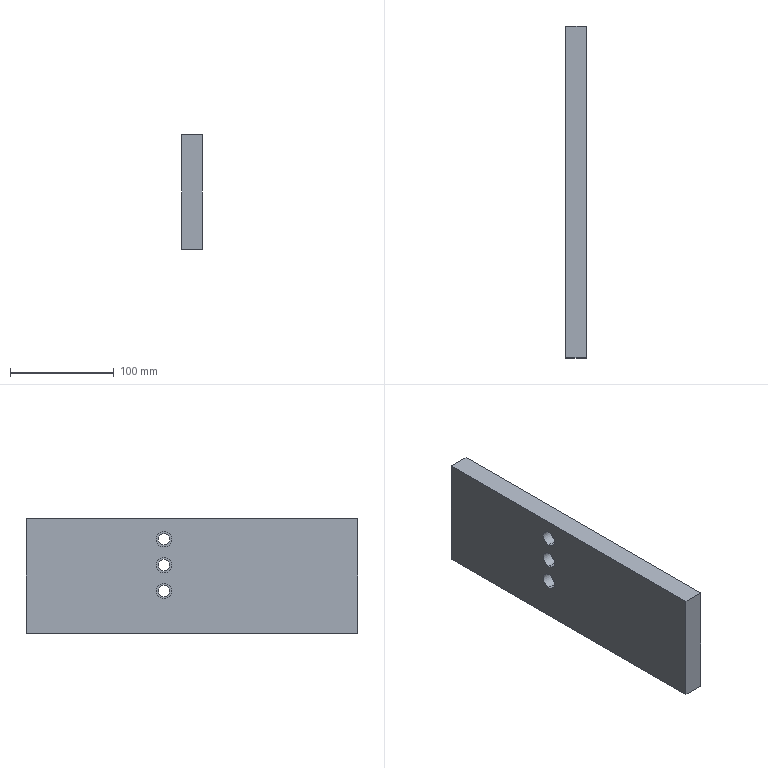Part | SolidWorks | features Extrusion 1, HoleWzd 1 | 1 solid | 21 faces | box 20 x 320 x 110 mm | volume 695848 mm3 | cylinder 12 | plane 9 | commonest cylinder face diameters 11 x6 15 x6
STEP:
#1=CARTESIAN_POINT('',(-110.,327.,32.99));
#2=VERTEX_POINT('',#1);
#3=CARTESIAN_POINT('',(-110.,327.,47.99));
#4=VERTEX_POINT('',#3);
#5=CARTESIAN_POINT('',(-110.,327.,40.49));
#6=DIRECTION('',(-1.,0.,0.));
#7=DIRECTION('',(0.,0.,1.));
#8=AXIS2_PLACEMENT_3D('',#5,#6,#7);
#9=CIRCLE('',#8,7.5);
#10=EDGE_CURVE('',#2,#4,#9,.T.);
#11=ORIENTED_EDGE('',*,*,#10,.F.);
#12=CARTESIAN_POINT('',(-120.,327.,32.99));
#13=VERTEX_POINT('',#12);
#14=CARTESIAN_POINT('',(-120.,327.,32.99));
#15=DIRECTION('',(-1.,0.,0.));
#16=VECTOR('',#15,1000.);
#17=LINE('',#14,#16);
#18=EDGE_CURVE('',#2,#13,#17,.T.);
#19=ORIENTED_EDGE('',*,*,#18,.T.);
#20=CARTESIAN_POINT('',(-120.,327.,47.99));
#21=VERTEX_POINT('',#20);
#22=CARTESIAN_POINT('',(-120.,327.,40.49));
#23=DIRECTION('',(-1.,0.,0.));
#24=DIRECTION('',(0.,0.,1.));
#25=AXIS2_PLACEMENT_3D('',#22,#23,#24);
#26=CIRCLE('',#25,7.5);
#27=EDGE_CURVE('',#13,#21,#26,.T.);
#28=ORIENTED_EDGE('',*,*,#27,.T.);
#29=CARTESIAN_POINT('',(-120.,327.,47.99));
#30=DIRECTION('',(-1.,0.,0.));
#31=VECTOR('',#30,1000.);
#32=LINE('',#29,#31);
#33=EDGE_CURVE('',#4,#21,#32,.T.);
#34=ORIENTED_EDGE('',*,*,#33,.F.);
#35=EDGE_LOOP('',(#11,#19,#28,#34));
#36=FACE_OUTER_BOUND('',#35,.T.);
#37=CARTESIAN_POINT('',(-120.,327.,40.49));
#38=DIRECTION('',(-1.,0.,0.));
#39=DIRECTION('',(0.,0.,1.));
#40=AXIS2_PLACEMENT_3D('',#37,#38,#39);
#41=CYLINDRICAL_SURFACE('',#40,7.5);
#42=ADVANCED_FACE('',(#36),#41,.F.);
#43=CARTESIAN_POINT('',(-100.,327.,45.99));
#44=VERTEX_POINT('',#43);
#45=CARTESIAN_POINT('',(-100.,327.,34.99));
#46=VERTEX_POINT('',#45);
#47=CARTESIAN_POINT('',(-100.,327.,40.49));
#48=DIRECTION('',(1.,0.,0.));
#49=DIRECTION('',(0.,1.,0.));
#50=AXIS2_PLACEMENT_3D('',#47,#48,#49);
#51=CIRCLE('',#50,5.5);
#52=EDGE_CURVE('',#44,#46,#51,.T.);
#53=ORIENTED_EDGE('',*,*,#52,.T.);
#54=CARTESIAN_POINT('',(-110.,327.,34.99));
#55=VERTEX_POINT('',#54);
#56=CARTESIAN_POINT('',(-120.,327.,34.99));
#57=DIRECTION('',(-1.,0.,0.));
#58=VECTOR('',#57,1000.);
#59=LINE('',#56,#58);
#60=EDGE_CURVE('',#46,#55,#59,.T.);
#61=ORIENTED_EDGE('',*,*,#60,.T.);
#62=CARTESIAN_POINT('',(-110.,327.,45.99));
#63=VERTEX_POINT('',#62);
#64=CARTESIAN_POINT('',(-110.,327.,40.49));
#65=DIRECTION('',(-1.,0.,0.));
#66=DIRECTION('',(0.,0.,1.));
#67=AXIS2_PLACEMENT_3D('',#64,#65,#66);
#68=CIRCLE('',#67,5.5);
#69=EDGE_CURVE('',#55,#63,#68,.T.);
#70=ORIENTED_EDGE('',*,*,#69,.T.);
#71=CARTESIAN_POINT('',(-120.,327.,45.99));
#72=DIRECTION('',(-1.,0.,0.));
#73=VECTOR('',#72,1000.);
#74=LINE('',#71,#73);
#75=EDGE_CURVE('',#44,#63,#74,.T.);
#76=ORIENTED_EDGE('',*,*,#75,.F.);
#77=EDGE_LOOP('',(#53,#61,#70,#76));
#78=FACE_OUTER_BOUND('',#77,.T.);
#79=CARTESIAN_POINT('',(-120.,327.,40.49));
#80=DIRECTION('',(-1.,0.,0.));
#81=DIRECTION('',(0.,0.,1.));
#82=AXIS2_PLACEMENT_3D('',#79,#80,#81);
#83=CYLINDRICAL_SURFACE('',#82,5.5);
#84=ADVANCED_FACE('',(#78),#83,.F.);
#85=CARTESIAN_POINT('',(-110.,327.,57.99));
#86=VERTEX_POINT('',#85);
#87=CARTESIAN_POINT('',(-110.,327.,72.99));
#88=VERTEX_POINT('',#87);
#89=CARTESIAN_POINT('',(-110.,327.,65.49));
#90=DIRECTION('',(-1.,0.,0.));
#91=DIRECTION('',(0.,0.,1.));
#92=AXIS2_PLACEMENT_3D('',#89,#90,#91);
#93=CIRCLE('',#92,7.5);
#94=EDGE_CURVE('',#86,#88,#93,.T.);
#95=ORIENTED_EDGE('',*,*,#94,.F.);
#96=CARTESIAN_POINT('',(-120.,327.,57.99));
#97=VERTEX_POINT('',#96);
#98=CARTESIAN_POINT('',(-120.,327.,57.99));
#99=DIRECTION('',(-1.,0.,0.));
#100=VECTOR('',#99,1000.);
#101=LINE('',#98,#100);
#102=EDGE_CURVE('',#86,#97,#101,.T.);
#103=ORIENTED_EDGE('',*,*,#102,.T.);
#104=CARTESIAN_POINT('',(-120.,327.,72.99));
#105=VERTEX_POINT('',#104);
#106=CARTESIAN_POINT('',(-120.,327.,65.49));
#107=DIRECTION('',(-1.,0.,0.));
#108=DIRECTION('',(0.,0.,1.));
#109=AXIS2_PLACEMENT_3D('',#106,#107,#108);
#110=CIRCLE('',#109,7.5);
#111=EDGE_CURVE('',#97,#105,#110,.T.);
#112=ORIENTED_EDGE('',*,*,#111,.T.);
#113=CARTESIAN_POINT('',(-120.,327.,72.99));
#114=DIRECTION('',(-1.,0.,0.));
#115=VECTOR('',#114,1000.);
#116=LINE('',#113,#115);
#117=EDGE_CURVE('',#88,#105,#116,.T.);
#118=ORIENTED_EDGE('',*,*,#117,.F.);
#119=EDGE_LOOP('',(#95,#103,#112,#118));
#120=FACE_OUTER_BOUND('',#119,.T.);
#121=CARTESIAN_POINT('',(-120.,327.,65.49));
#122=DIRECTION('',(-1.,0.,0.));
#123=DIRECTION('',(0.,0.,1.));
#124=AXIS2_PLACEMENT_3D('',#121,#122,#123);
#125=CYLINDRICAL_SURFACE('',#124,7.5);
#126=ADVANCED_FACE('',(#120),#125,.F.);
#127=CARTESIAN_POINT('',(-100.,327.,70.99));
#128=VERTEX_POINT('',#127);
#129=CARTESIAN_POINT('',(-100.,327.,59.99));
#130=VERTEX_POINT('',#129);
#131=CARTESIAN_POINT('',(-100.,327.,65.49));
#132=DIRECTION('',(1.,0.,0.));
#133=DIRECTION('',(0.,1.,0.));
#134=AXIS2_PLACEMENT_3D('',#131,#132,#133);
#135=CIRCLE('',#134,5.5);
#136=EDGE_CURVE('',#128,#130,#135,.T.);
#137=ORIENTED_EDGE('',*,*,#136,.T.);
#138=CARTESIAN_POINT('',(-110.,327.,59.99));
#139=VERTEX_POINT('',#138);
#140=CARTESIAN_POINT('',(-120.,327.,59.99));
#141=DIRECTION('',(-1.,0.,0.));
#142=VECTOR('',#141,1000.);
#143=LINE('',#140,#142);
#144=EDGE_CURVE('',#130,#139,#143,.T.);
#145=ORIENTED_EDGE('',*,*,#144,.T.);
#146=CARTESIAN_POINT('',(-110.,327.,70.99));
#147=VERTEX_POINT('',#146);
#148=CARTESIAN_POINT('',(-110.,327.,65.49));
#149=DIRECTION('',(-1.,0.,0.));
#150=DIRECTION('',(0.,0.,1.));
#151=AXIS2_PLACEMENT_3D('',#148,#149,#150);
#152=CIRCLE('',#151,5.5);
#153=EDGE_CURVE('',#139,#147,#152,.T.);
#154=ORIENTED_EDGE('',*,*,#153,.T.);
#155=CARTESIAN_POINT('',(-120.,327.,70.99));
#156=DIRECTION('',(-1.,0.,0.));
#157=VECTOR('',#156,1000.);
#158=LINE('',#155,#157);
#159=EDGE_CURVE('',#128,#147,#158,.T.);
#160=ORIENTED_EDGE('',*,*,#159,.F.);
#161=EDGE_LOOP('',(#137,#145,#154,#160));
#162=FACE_OUTER_BOUND('',#161,.T.);
#163=CARTESIAN_POINT('',(-120.,327.,65.49));
#164=DIRECTION('',(-1.,0.,0.));
#165=DIRECTION('',(0.,0.,1.));
#166=AXIS2_PLACEMENT_3D('',#163,#164,#165);
#167=CYLINDRICAL_SURFACE('',#166,5.5);
#168=ADVANCED_FACE('',(#162),#167,.F.);
#169=CARTESIAN_POINT('',(-110.,327.,82.99));
#170=VERTEX_POINT('',#169);
#171=CARTESIAN_POINT('',(-110.,327.,97.99));
#172=VERTEX_POINT('',#171);
#173=CARTESIAN_POINT('',(-110.,327.,90.49));
#174=DIRECTION('',(-1.,0.,0.));
#175=DIRECTION('',(0.,0.,1.));
#176=AXIS2_PLACEMENT_3D('',#173,#174,#175);
#177=CIRCLE('',#176,7.5);
#178=EDGE_CURVE('',#170,#172,#177,.T.);
#179=ORIENTED_EDGE('',*,*,#178,.F.);
#180=CARTESIAN_POINT('',(-120.,327.,82.99));
#181=VERTEX_POINT('',#180);
#182=CARTESIAN_POINT('',(-120.,327.,82.99));
#183=DIRECTION('',(-1.,0.,0.));
#184=VECTOR('',#183,1000.);
#185=LINE('',#182,#184);
#186=EDGE_CURVE('',#170,#181,#185,.T.);
#187=ORIENTED_EDGE('',*,*,#186,.T.);
#188=CARTESIAN_POINT('',(-120.,327.,97.99));
#189=VERTEX_POINT('',#188);
#190=CARTESIAN_POINT('',(-120.,327.,90.49));
#191=DIRECTION('',(-1.,0.,0.));
#192=DIRECTION('',(0.,0.,1.));
#193=AXIS2_PLACEMENT_3D('',#190,#191,#192);
#194=CIRCLE('',#193,7.5);
#195=EDGE_CURVE('',#181,#189,#194,.T.);
#196=ORIENTED_EDGE('',*,*,#195,.T.);
#197=CARTESIAN_POINT('',(-120.,327.,97.99));
#198=DIRECTION('',(-1.,0.,0.));
#199=VECTOR('',#198,1000.);
#200=LINE('',#197,#199);
#201=EDGE_CURVE('',#172,#189,#200,.T.);
#202=ORIENTED_EDGE('',*,*,#201,.F.);
#203=EDGE_LOOP('',(#179,#187,#196,#202));
#204=FACE_OUTER_BOUND('',#203,.T.);
#205=CARTESIAN_POINT('',(-120.,327.,90.49));
#206=DIRECTION('',(-1.,0.,0.));
#207=DIRECTION('',(0.,0.,1.));
#208=AXIS2_PLACEMENT_3D('',#205,#206,#207);
#209=CYLINDRICAL_SURFACE('',#208,7.5);
#210=ADVANCED_FACE('',(#204),#209,.F.);
#211=CARTESIAN_POINT('',(-100.,327.,95.99));
#212=VERTEX_POINT('',#211);
#213=CARTESIAN_POINT('',(-100.,327.,84.99));
#214=VERTEX_POINT('',#213);
#215=CARTESIAN_POINT('',(-100.,327.,90.49));
#216=DIRECTION('',(1.,0.,0.));
#217=DIRECTION('',(0.,1.,0.));
#218=AXIS2_PLACEMENT_3D('',#215,#216,#217);
#219=CIRCLE('',#218,5.5);
#220=EDGE_CURVE('',#212,#214,#219,.T.);
#221=ORIENTED_EDGE('',*,*,#220,.T.);
#222=CARTESIAN_POINT('',(-110.,327.,84.99));
#223=VERTEX_POINT('',#222);
#224=CARTESIAN_POINT('',(-120.,327.,84.99));
#225=DIRECTION('',(-1.,0.,0.));
#226=VECTOR('',#225,1000.);
#227=LINE('',#224,#226);
#228=EDGE_CURVE('',#214,#223,#227,.T.);
#229=ORIENTED_EDGE('',*,*,#228,.T.);
#230=CARTESIAN_POINT('',(-110.,327.,95.99));
#231=VERTEX_POINT('',#230);
#232=CARTESIAN_POINT('',(-110.,327.,90.49));
#233=DIRECTION('',(-1.,0.,0.));
#234=DIRECTION('',(0.,0.,1.));
#235=AXIS2_PLACEMENT_3D('',#232,#233,#234);
#236=CIRCLE('',#235,5.5);
#237=EDGE_CURVE('',#223,#231,#236,.T.);
#238=ORIENTED_EDGE('',*,*,#237,.T.);
#239=CARTESIAN_POINT('',(-120.,327.,95.99));
#240=DIRECTION('',(-1.,0.,0.));
#241=VECTOR('',#240,1000.);
#242=LINE('',#239,#241);
#243=EDGE_CURVE('',#212,#231,#242,.T.);
#244=ORIENTED_EDGE('',*,*,#243,.F.);
#245=EDGE_LOOP('',(#221,#229,#238,#244));
#246=FACE_OUTER_BOUND('',#245,.T.);
#247=CARTESIAN_POINT('',(-120.,327.,90.49));
#248=DIRECTION('',(-1.,0.,0.));
#249=DIRECTION('',(0.,0.,1.));
#250=AXIS2_PLACEMENT_3D('',#247,#248,#249);
#251=CYLINDRICAL_SURFACE('',#250,5.5);
#252=ADVANCED_FACE('',(#246),#251,.F.);
#253=CARTESIAN_POINT('',(-120.,460.,0.));
#254=VERTEX_POINT('',#253);
#255=CARTESIAN_POINT('',(-100.,460.,0.));
#256=VERTEX_POINT('',#255);
#257=CARTESIAN_POINT('',(-120.,460.,0.));
#258=DIRECTION('',(1.,0.,0.));
#259=VECTOR('',#258,1000.);
#260=LINE('',#257,#259);
#261=EDGE_CURVE('',#254,#256,#260,.T.);
#262=ORIENTED_EDGE('',*,*,#261,.F.);
#263=CARTESIAN_POINT('',(-120.,460.,110.));
#264=VERTEX_POINT('',#263);
#265=CARTESIAN_POINT('',(-120.,460.,110.));
#266=DIRECTION('',(0.,0.,-1.));
#267=VECTOR('',#266,1000.);
#268=LINE('',#265,#267);
#269=EDGE_CURVE('',#264,#254,#268,.T.);
#270=ORIENTED_EDGE('',*,*,#269,.F.);
#271=CARTESIAN_POINT('',(-100.,460.,110.));
#272=VERTEX_POINT('',#271);
#273=CARTESIAN_POINT('',(-120.,460.,110.));
#274=DIRECTION('',(1.,0.,0.));
#275=VECTOR('',#274,1000.);
#276=LINE('',#273,#275);
#277=EDGE_CURVE('',#264,#272,#276,.T.);
#278=ORIENTED_EDGE('',*,*,#277,.T.);
#279=CARTESIAN_POINT('',(-100.,460.,110.));
#280=DIRECTION('',(0.,0.,-1.));
#281=VECTOR('',#280,1000.);
#282=LINE('',#279,#281);
#283=EDGE_CURVE('',#272,#256,#282,.T.);
#284=ORIENTED_EDGE('',*,*,#283,.T.);
#285=EDGE_LOOP('',(#262,#270,#278,#284));
#286=FACE_OUTER_BOUND('',#285,.T.);
#287=CARTESIAN_POINT('',(-120.,460.,110.));
#288=DIRECTION('',(0.,1.,0.));
#289=DIRECTION('',(0.,0.,1.));
#290=AXIS2_PLACEMENT_3D('',#287,#288,#289);
#291=PLANE('',#290);
#292=ADVANCED_FACE('',(#286),#291,.T.);
#293=CARTESIAN_POINT('',(-120.,327.,40.49));
#294=DIRECTION('',(-1.,0.,0.));
#295=DIRECTION('',(0.,0.,1.));
#296=AXIS2_PLACEMENT_3D('',#293,#294,#295);
#297=CIRCLE('',#296,7.5);
#298=EDGE_CURVE('',#21,#13,#297,.T.);
#299=ORIENTED_EDGE('',*,*,#298,.F.);
#300=ORIENTED_EDGE('',*,*,#27,.F.);
#301=EDGE_LOOP('',(#299,#300));
#302=FACE_BOUND('',#301,.T.);
#303=CARTESIAN_POINT('',(-120.,327.,65.49));
#304=DIRECTION('',(-1.,0.,0.));
#305=DIRECTION('',(0.,0.,1.));
#306=AXIS2_PLACEMENT_3D('',#303,#304,#305);
#307=CIRCLE('',#306,7.5);
#308=EDGE_CURVE('',#105,#97,#307,.T.);
#309=ORIENTED_EDGE('',*,*,#308,.F.);
#310=ORIENTED_EDGE('',*,*,#111,.F.);
#311=EDGE_LOOP('',(#309,#310));
#312=FACE_BOUND('',#311,.T.);
#313=CARTESIAN_POINT('',(-120.,327.,90.49));
#314=DIRECTION('',(-1.,0.,0.));
#315=DIRECTION('',(0.,0.,1.));
#316=AXIS2_PLACEMENT_3D('',#313,#314,#315);
#317=CIRCLE('',#316,7.5);
#318=EDGE_CURVE('',#189,#181,#317,.T.);
#319=ORIENTED_EDGE('',*,*,#318,.F.);
#320=ORIENTED_EDGE('',*,*,#195,.F.);
#321=EDGE_LOOP('',(#319,#320));
#322=FACE_BOUND('',#321,.T.);
#323=CARTESIAN_POINT('',(-120.,140.,0.));
#324=VERTEX_POINT('',#323);
#325=CARTESIAN_POINT('',(-120.,460.,0.));
#326=DIRECTION('',(0.,-1.,0.));
#327=VECTOR('',#326,1000.);
#328=LINE('',#325,#327);
#329=EDGE_CURVE('',#254,#324,#328,.T.);
#330=ORIENTED_EDGE('',*,*,#329,.T.);
#331=CARTESIAN_POINT('',(-120.,140.,110.));
#332=VERTEX_POINT('',#331);
#333=CARTESIAN_POINT('',(-120.,140.,110.));
#334=DIRECTION('',(0.,0.,-1.));
#335=VECTOR('',#334,1000.);
#336=LINE('',#333,#335);
#337=EDGE_CURVE('',#332,#324,#336,.T.);
#338=ORIENTED_EDGE('',*,*,#337,.F.);
#339=CARTESIAN_POINT('',(-120.,460.,110.));
#340=DIRECTION('',(0.,-1.,0.));
#341=VECTOR('',#340,1000.);
#342=LINE('',#339,#341);
#343=EDGE_CURVE('',#264,#332,#342,.T.);
#344=ORIENTED_EDGE('',*,*,#343,.F.);
#345=ORIENTED_EDGE('',*,*,#269,.T.);
#346=EDGE_LOOP('',(#330,#338,#344,#345));
#347=FACE_OUTER_BOUND('',#346,.T.);
#348=CARTESIAN_POINT('',(-120.,460.,110.));
#349=DIRECTION('',(1.,0.,0.));
#350=DIRECTION('',(0.,1.,0.));
#351=AXIS2_PLACEMENT_3D('',#348,#349,#350);
#352=PLANE('',#351);
#353=ADVANCED_FACE('',(#302,#312,#322,#347),#352,.F.);
#354=CARTESIAN_POINT('',(-100.,140.,0.));
#355=VERTEX_POINT('',#354);
#356=CARTESIAN_POINT('',(-120.,140.,0.));
#357=DIRECTION('',(1.,0.,0.));
#358=VECTOR('',#357,1000.);
#359=LINE('',#356,#358);
#360=EDGE_CURVE('',#324,#355,#359,.T.);
#361=ORIENTED_EDGE('',*,*,#360,.T.);
#362=CARTESIAN_POINT('',(-100.,140.,110.));
#363=VERTEX_POINT('',#362);
#364=CARTESIAN_POINT('',(-100.,140.,110.));
#365=DIRECTION('',(0.,0.,-1.));
#366=VECTOR('',#365,1000.);
#367=LINE('',#364,#366);
#368=EDGE_CURVE('',#363,#355,#367,.T.);
#369=ORIENTED_EDGE('',*,*,#368,.F.);
#370=CARTESIAN_POINT('',(-120.,140.,110.));
#371=DIRECTION('',(1.,0.,0.));
#372=VECTOR('',#371,1000.);
#373=LINE('',#370,#372);
#374=EDGE_CURVE('',#332,#363,#373,.T.);
#375=ORIENTED_EDGE('',*,*,#374,.F.);
#376=ORIENTED_EDGE('',*,*,#337,.T.);
#377=EDGE_LOOP('',(#361,#369,#375,#376));
#378=FACE_OUTER_BOUND('',#377,.T.);
#379=CARTESIAN_POINT('',(-120.,140.,110.));
#380=DIRECTION('',(0.,1.,0.));
#381=DIRECTION('',(0.,0.,1.));
#382=AXIS2_PLACEMENT_3D('',#379,#380,#381);
#383=PLANE('',#382);
#384=ADVANCED_FACE('',(#378),#383,.F.);
#385=ORIENTED_EDGE('',*,*,#52,.F.);
#386=CARTESIAN_POINT('',(-100.,327.,40.49));
#387=DIRECTION('',(1.,0.,0.));
#388=DIRECTION('',(0.,1.,0.));
#389=AXIS2_PLACEMENT_3D('',#386,#387,#388);
#390=CIRCLE('',#389,5.5);
#391=EDGE_CURVE('',#46,#44,#390,.T.);
#392=ORIENTED_EDGE('',*,*,#391,.F.);
#393=EDGE_LOOP('',(#385,#392));
#394=FACE_BOUND('',#393,.T.);
#395=ORIENTED_EDGE('',*,*,#136,.F.);
#396=CARTESIAN_POINT('',(-100.,327.,65.49));
#397=DIRECTION('',(1.,0.,0.));
#398=DIRECTION('',(0.,1.,0.));
#399=AXIS2_PLACEMENT_3D('',#396,#397,#398);
#400=CIRCLE('',#399,5.5);
#401=EDGE_CURVE('',#130,#128,#400,.T.);
#402=ORIENTED_EDGE('',*,*,#401,.F.);
#403=EDGE_LOOP('',(#395,#402));
#404=FACE_BOUND('',#403,.T.);
#405=ORIENTED_EDGE('',*,*,#220,.F.);
#406=CARTESIAN_POINT('',(-100.,327.,90.49));
#407=DIRECTION('',(1.,0.,0.));
#408=DIRECTION('',(0.,1.,0.));
#409=AXIS2_PLACEMENT_3D('',#406,#407,#408);
#410=CIRCLE('',#409,5.5);
#411=EDGE_CURVE('',#214,#212,#410,.T.);
#412=ORIENTED_EDGE('',*,*,#411,.F.);
#413=EDGE_LOOP('',(#405,#412));
#414=FACE_BOUND('',#413,.T.);
#415=CARTESIAN_POINT('',(-100.,460.,0.));
#416=DIRECTION('',(0.,-1.,0.));
#417=VECTOR('',#416,1000.);
#418=LINE('',#415,#417);
#419=EDGE_CURVE('',#256,#355,#418,.T.);
#420=ORIENTED_EDGE('',*,*,#419,.F.);
#421=ORIENTED_EDGE('',*,*,#283,.F.);
#422=CARTESIAN_POINT('',(-100.,460.,110.));
#423=DIRECTION('',(0.,-1.,0.));
#424=VECTOR('',#423,1000.);
#425=LINE('',#422,#424);
#426=EDGE_CURVE('',#272,#363,#425,.T.);
#427=ORIENTED_EDGE('',*,*,#426,.T.);
#428=ORIENTED_EDGE('',*,*,#368,.T.);
#429=EDGE_LOOP('',(#420,#421,#427,#428));
#430=FACE_OUTER_BOUND('',#429,.T.);
#431=CARTESIAN_POINT('',(-100.,460.,110.));
#432=DIRECTION('',(1.,0.,0.));
#433=DIRECTION('',(0.,1.,0.));
#434=AXIS2_PLACEMENT_3D('',#431,#432,#433);
#435=PLANE('',#434);
#436=ADVANCED_FACE('',(#394,#404,#414,#430),#435,.T.);
#437=ORIENTED_EDGE('',*,*,#277,.F.);
#438=ORIENTED_EDGE('',*,*,#343,.T.);
#439=ORIENTED_EDGE('',*,*,#374,.T.);
#440=ORIENTED_EDGE('',*,*,#426,.F.);
#441=EDGE_LOOP('',(#437,#438,#439,#440));
#442=FACE_OUTER_BOUND('',#441,.T.);
#443=CARTESIAN_POINT('',(0.,0.,110.));
#444=DIRECTION('',(0.,0.,-1.));
#445=DIRECTION('',(-1.,0.,0.));
#446=AXIS2_PLACEMENT_3D('',#443,#444,#445);
#447=PLANE('',#446);
#448=ADVANCED_FACE('',(#442),#447,.F.);
#449=ORIENTED_EDGE('',*,*,#261,.T.);
#450=ORIENTED_EDGE('',*,*,#419,.T.);
#451=ORIENTED_EDGE('',*,*,#360,.F.);
#452=ORIENTED_EDGE('',*,*,#329,.F.);
#453=EDGE_LOOP('',(#449,#450,#451,#452));
#454=FACE_OUTER_BOUND('',#453,.T.);
#455=CARTESIAN_POINT('',(0.,0.,0.));
#456=DIRECTION('',(0.,0.,-1.));
#457=DIRECTION('',(-1.,0.,0.));
#458=AXIS2_PLACEMENT_3D('',#455,#456,#457);
#459=PLANE('',#458);
#460=ADVANCED_FACE('',(#454),#459,.T.);
#461=ORIENTED_EDGE('',*,*,#228,.F.);
#462=ORIENTED_EDGE('',*,*,#411,.T.);
#463=ORIENTED_EDGE('',*,*,#243,.T.);
#464=CARTESIAN_POINT('',(-110.,327.,90.49));
#465=DIRECTION('',(-1.,0.,0.));
#466=DIRECTION('',(0.,0.,1.));
#467=AXIS2_PLACEMENT_3D('',#464,#465,#466);
#468=CIRCLE('',#467,5.5);
#469=EDGE_CURVE('',#231,#223,#468,.T.);
#470=ORIENTED_EDGE('',*,*,#469,.T.);
#471=EDGE_LOOP('',(#461,#462,#463,#470));
#472=FACE_OUTER_BOUND('',#471,.T.);
#473=CARTESIAN_POINT('',(-120.,327.,90.49));
#474=DIRECTION('',(-1.,0.,0.));
#475=DIRECTION('',(0.,0.,1.));
#476=AXIS2_PLACEMENT_3D('',#473,#474,#475);
#477=CYLINDRICAL_SURFACE('',#476,5.5);
#478=ADVANCED_FACE('',(#472),#477,.F.);
#479=ORIENTED_EDGE('',*,*,#469,.F.);
#480=ORIENTED_EDGE('',*,*,#237,.F.);
#481=EDGE_LOOP('',(#479,#480));
#482=FACE_BOUND('',#481,.T.);
#483=CARTESIAN_POINT('',(-110.,327.,90.49));
#484=DIRECTION('',(-1.,0.,0.));
#485=DIRECTION('',(0.,0.,1.));
#486=AXIS2_PLACEMENT_3D('',#483,#484,#485);
#487=CIRCLE('',#486,7.5);
#488=EDGE_CURVE('',#172,#170,#487,.T.);
#489=ORIENTED_EDGE('',*,*,#488,.T.);
#490=ORIENTED_EDGE('',*,*,#178,.T.);
#491=EDGE_LOOP('',(#489,#490));
#492=FACE_OUTER_BOUND('',#491,.T.);
#493=CARTESIAN_POINT('',(-110.,332.5,90.49));
#494=DIRECTION('',(1.,0.,0.));
#495=DIRECTION('',(0.,0.,-1.));
#496=AXIS2_PLACEMENT_3D('',#493,#494,#495);
#497=PLANE('',#496);
#498=ADVANCED_FACE('',(#482,#492),#497,.F.);
#499=ORIENTED_EDGE('',*,*,#186,.F.);
#500=ORIENTED_EDGE('',*,*,#488,.F.);
#501=ORIENTED_EDGE('',*,*,#201,.T.);
#502=ORIENTED_EDGE('',*,*,#318,.T.);
#503=EDGE_LOOP('',(#499,#500,#501,#502));
#504=FACE_OUTER_BOUND('',#503,.T.);
#505=CARTESIAN_POINT('',(-120.,327.,90.49));
#506=DIRECTION('',(-1.,0.,0.));
#507=DIRECTION('',(0.,0.,1.));
#508=AXIS2_PLACEMENT_3D('',#505,#506,#507);
#509=CYLINDRICAL_SURFACE('',#508,7.5);
#510=ADVANCED_FACE('',(#504),#509,.F.);
#511=ORIENTED_EDGE('',*,*,#144,.F.);
#512=ORIENTED_EDGE('',*,*,#401,.T.);
#513=ORIENTED_EDGE('',*,*,#159,.T.);
#514=CARTESIAN_POINT('',(-110.,327.,65.49));
#515=DIRECTION('',(-1.,0.,0.));
#516=DIRECTION('',(0.,0.,1.));
#517=AXIS2_PLACEMENT_3D('',#514,#515,#516);
#518=CIRCLE('',#517,5.5);
#519=EDGE_CURVE('',#147,#139,#518,.T.);
#520=ORIENTED_EDGE('',*,*,#519,.T.);
#521=EDGE_LOOP('',(#511,#512,#513,#520));
#522=FACE_OUTER_BOUND('',#521,.T.);
#523=CARTESIAN_POINT('',(-120.,327.,65.49));
#524=DIRECTION('',(-1.,0.,0.));
#525=DIRECTION('',(0.,0.,1.));
#526=AXIS2_PLACEMENT_3D('',#523,#524,#525);
#527=CYLINDRICAL_SURFACE('',#526,5.5);
#528=ADVANCED_FACE('',(#522),#527,.F.);
#529=ORIENTED_EDGE('',*,*,#519,.F.);
#530=ORIENTED_EDGE('',*,*,#153,.F.);
#531=EDGE_LOOP('',(#529,#530));
#532=FACE_BOUND('',#531,.T.);
#533=CARTESIAN_POINT('',(-110.,327.,65.49));
#534=DIRECTION('',(-1.,0.,0.));
#535=DIRECTION('',(0.,0.,1.));
#536=AXIS2_PLACEMENT_3D('',#533,#534,#535);
#537=CIRCLE('',#536,7.5);
#538=EDGE_CURVE('',#88,#86,#537,.T.);
#539=ORIENTED_EDGE('',*,*,#538,.T.);
#540=ORIENTED_EDGE('',*,*,#94,.T.);
#541=EDGE_LOOP('',(#539,#540));
#542=FACE_OUTER_BOUND('',#541,.T.);
#543=CARTESIAN_POINT('',(-110.,332.5,65.49));
#544=DIRECTION('',(1.,0.,0.));
#545=DIRECTION('',(0.,0.,-1.));
#546=AXIS2_PLACEMENT_3D('',#543,#544,#545);
#547=PLANE('',#546);
#548=ADVANCED_FACE('',(#532,#542),#547,.F.);
#549=ORIENTED_EDGE('',*,*,#102,.F.);
#550=ORIENTED_EDGE('',*,*,#538,.F.);
#551=ORIENTED_EDGE('',*,*,#117,.T.);
#552=ORIENTED_EDGE('',*,*,#308,.T.);
#553=EDGE_LOOP('',(#549,#550,#551,#552));
#554=FACE_OUTER_BOUND('',#553,.T.);
#555=CARTESIAN_POINT('',(-120.,327.,65.49));
#556=DIRECTION('',(-1.,0.,0.));
#557=DIRECTION('',(0.,0.,1.));
#558=AXIS2_PLACEMENT_3D('',#555,#556,#557);
#559=CYLINDRICAL_SURFACE('',#558,7.5);
#560=ADVANCED_FACE('',(#554),#559,.F.);
#561=ORIENTED_EDGE('',*,*,#60,.F.);
#562=ORIENTED_EDGE('',*,*,#391,.T.);
#563=ORIENTED_EDGE('',*,*,#75,.T.);
#564=CARTESIAN_POINT('',(-110.,327.,40.49));
#565=DIRECTION('',(-1.,0.,0.));
#566=DIRECTION('',(0.,0.,1.));
#567=AXIS2_PLACEMENT_3D('',#564,#565,#566);
#568=CIRCLE('',#567,5.5);
#569=EDGE_CURVE('',#63,#55,#568,.T.);
#570=ORIENTED_EDGE('',*,*,#569,.T.);
#571=EDGE_LOOP('',(#561,#562,#563,#570));
#572=FACE_OUTER_BOUND('',#571,.T.);
#573=CARTESIAN_POINT('',(-120.,327.,40.49));
#574=DIRECTION('',(-1.,0.,0.));
#575=DIRECTION('',(0.,0.,1.));
#576=AXIS2_PLACEMENT_3D('',#573,#574,#575);
#577=CYLINDRICAL_SURFACE('',#576,5.5);
#578=ADVANCED_FACE('',(#572),#577,.F.);
#579=ORIENTED_EDGE('',*,*,#569,.F.);
#580=ORIENTED_EDGE('',*,*,#69,.F.);
#581=EDGE_LOOP('',(#579,#580));
#582=FACE_BOUND('',#581,.T.);
#583=CARTESIAN_POINT('',(-110.,327.,40.49));
#584=DIRECTION('',(-1.,0.,0.));
#585=DIRECTION('',(0.,0.,1.));
#586=AXIS2_PLACEMENT_3D('',#583,#584,#585);
#587=CIRCLE('',#586,7.5);
#588=EDGE_CURVE('',#4,#2,#587,.T.);
#589=ORIENTED_EDGE('',*,*,#588,.T.);
#590=ORIENTED_EDGE('',*,*,#10,.T.);
#591=EDGE_LOOP('',(#589,#590));
#592=FACE_OUTER_BOUND('',#591,.T.);
#593=CARTESIAN_POINT('',(-110.,332.5,40.49));
#594=DIRECTION('',(1.,0.,0.));
#595=DIRECTION('',(0.,0.,-1.));
#596=AXIS2_PLACEMENT_3D('',#593,#594,#595);
#597=PLANE('',#596);
#598=ADVANCED_FACE('',(#582,#592),#597,.F.);
#599=ORIENTED_EDGE('',*,*,#18,.F.);
#600=ORIENTED_EDGE('',*,*,#588,.F.);
#601=ORIENTED_EDGE('',*,*,#33,.T.);
#602=ORIENTED_EDGE('',*,*,#298,.T.);
#603=EDGE_LOOP('',(#599,#600,#601,#602));
#604=FACE_OUTER_BOUND('',#603,.T.);
#605=CARTESIAN_POINT('',(-120.,327.,40.49));
#606=DIRECTION('',(-1.,0.,0.));
#607=DIRECTION('',(0.,0.,1.));
#608=AXIS2_PLACEMENT_3D('',#605,#606,#607);
#609=CYLINDRICAL_SURFACE('',#608,7.5);
#610=ADVANCED_FACE('',(#604),#609,.F.);
#611=CLOSED_SHELL('',(#42,#84,#126,#168,#210,#252,#292,#353,#384,#436,#448,#460,#478,#498,#510,#528,#548,#560,#578,#598,#610));
#612=MANIFOLD_SOLID_BREP('',#611);
#613=CARTESIAN_POINT('',(0.,0.,0.));
#614=DIRECTION('',(0.,0.,1.));
#615=DIRECTION('',(1.,0.,0.));
#616=AXIS2_PLACEMENT_3D('',#613,#614,#615);
#617=(LENGTH_UNIT()NAMED_UNIT(*)SI_UNIT(.MILLI.,.METRE.));
#618=UNCERTAINTY_MEASURE_WITH_UNIT(LENGTH_MEASURE(0.00001),#617,'','');
#619=(NAMED_UNIT(*)PLANE_ANGLE_UNIT()SI_UNIT($,.RADIAN.));
#620=(NAMED_UNIT(*)SI_UNIT($,.STERADIAN.)SOLID_ANGLE_UNIT());
#621=(GEOMETRIC_REPRESENTATION_CONTEXT(3)GLOBAL_UNCERTAINTY_ASSIGNED_CONTEXT((#618))GLOBAL_UNIT_ASSIGNED_CONTEXT((#617,#619,#620))REPRESENTATION_CONTEXT('',''));
#622=ADVANCED_BREP_SHAPE_REPRESENTATION('',(#612,#616),#621);